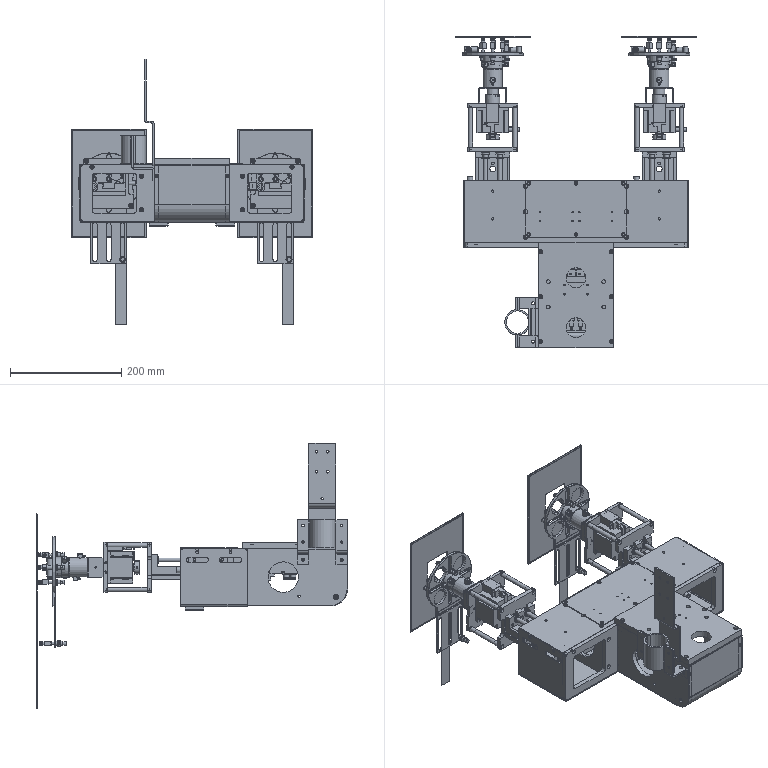Part | NX | 125 solids | 5714 faces | volume 3304719 mm3 | plane 2984 | cylinder 1390 | cone 846 | spline 444 | torus 50 | commonest cylinder face diameters 10 x98 2.5 x92 3.3 x92 7 x86 8 x74 4.5 x72